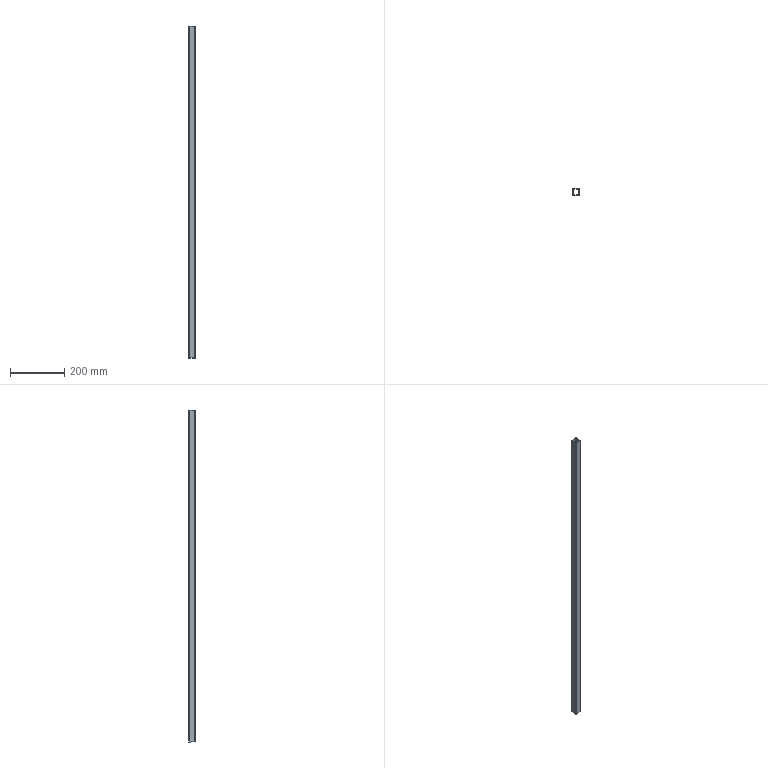Part | SolidWorks | features Extrusion 1 | 1 solid | 18 faces | box 25 x 25 x 1224 mm | volume 212608 mm3 | plane 10 | cylinder 8 | commonest cylinder face diameters 4 x4 8 x4
STEP:
#1=CARTESIAN_POINT('',(12.5,8.5,1224.));
#2=VERTEX_POINT('',#1);
#3=CARTESIAN_POINT('',(8.5,12.5,1224.));
#4=VERTEX_POINT('',#3);
#5=CARTESIAN_POINT('',(8.5,8.5,1224.));
#6=DIRECTION('',(0.,0.,1.));
#7=DIRECTION('',(1.,0.,0.));
#8=AXIS2_PLACEMENT_3D('',#5,#6,#7);
#9=CIRCLE('',#8,4.);
#10=EDGE_CURVE('',#2,#4,#9,.T.);
#11=ORIENTED_EDGE('',*,*,#10,.T.);
#12=CARTESIAN_POINT('',(-8.5,12.5,1224.));
#13=VERTEX_POINT('',#12);
#14=CARTESIAN_POINT('',(8.5,12.5,1224.));
#15=DIRECTION('',(-1.,0.,0.));
#16=VECTOR('',#15,1000.);
#17=LINE('',#14,#16);
#18=EDGE_CURVE('',#4,#13,#17,.T.);
#19=ORIENTED_EDGE('',*,*,#18,.T.);
#20=CARTESIAN_POINT('',(-12.5,8.5,1224.));
#21=VERTEX_POINT('',#20);
#22=CARTESIAN_POINT('',(-8.5,8.5,1224.));
#23=DIRECTION('',(0.,0.,1.));
#24=DIRECTION('',(1.,0.,0.));
#25=AXIS2_PLACEMENT_3D('',#22,#23,#24);
#26=CIRCLE('',#25,4.);
#27=EDGE_CURVE('',#13,#21,#26,.T.);
#28=ORIENTED_EDGE('',*,*,#27,.T.);
#29=CARTESIAN_POINT('',(-12.5,-8.5,1224.));
#30=VERTEX_POINT('',#29);
#31=CARTESIAN_POINT('',(-12.5,-8.5,1224.));
#32=DIRECTION('',(0.,-1.,0.));
#33=VECTOR('',#32,1000.);
#34=LINE('',#31,#33);
#35=EDGE_CURVE('',#21,#30,#34,.T.);
#36=ORIENTED_EDGE('',*,*,#35,.T.);
#37=CARTESIAN_POINT('',(-8.5,-12.5,1224.));
#38=VERTEX_POINT('',#37);
#39=CARTESIAN_POINT('',(-8.5,-8.5,1224.));
#40=DIRECTION('',(0.,0.,1.));
#41=DIRECTION('',(1.,0.,0.));
#42=AXIS2_PLACEMENT_3D('',#39,#40,#41);
#43=CIRCLE('',#42,4.);
#44=EDGE_CURVE('',#30,#38,#43,.T.);
#45=ORIENTED_EDGE('',*,*,#44,.T.);
#46=CARTESIAN_POINT('',(8.5,-12.5,1224.));
#47=VERTEX_POINT('',#46);
#48=CARTESIAN_POINT('',(-8.5,-12.5,1224.));
#49=DIRECTION('',(1.,0.,0.));
#50=VECTOR('',#49,1000.);
#51=LINE('',#48,#50);
#52=EDGE_CURVE('',#38,#47,#51,.T.);
#53=ORIENTED_EDGE('',*,*,#52,.T.);
#54=CARTESIAN_POINT('',(12.5,-8.5,1224.));
#55=VERTEX_POINT('',#54);
#56=CARTESIAN_POINT('',(8.5,-8.5,1224.));
#57=DIRECTION('',(0.,0.,1.));
#58=DIRECTION('',(1.,0.,0.));
#59=AXIS2_PLACEMENT_3D('',#56,#57,#58);
#60=CIRCLE('',#59,4.);
#61=EDGE_CURVE('',#47,#55,#60,.T.);
#62=ORIENTED_EDGE('',*,*,#61,.T.);
#63=CARTESIAN_POINT('',(12.5,8.5,1224.));
#64=DIRECTION('',(0.,1.,0.));
#65=VECTOR('',#64,1000.);
#66=LINE('',#63,#65);
#67=EDGE_CURVE('',#55,#2,#66,.T.);
#68=ORIENTED_EDGE('',*,*,#67,.T.);
#69=EDGE_LOOP('',(#11,#19,#28,#36,#45,#53,#62,#68));
#70=FACE_OUTER_BOUND('',#69,.T.);
#71=CARTESIAN_POINT('',(-10.5,8.5,1224.));
#72=VERTEX_POINT('',#71);
#73=CARTESIAN_POINT('',(-10.5,-8.5,1224.));
#74=VERTEX_POINT('',#73);
#75=CARTESIAN_POINT('',(-10.5,-8.5,1224.));
#76=DIRECTION('',(0.,-1.,0.));
#77=VECTOR('',#76,1000.);
#78=LINE('',#75,#77);
#79=EDGE_CURVE('',#72,#74,#78,.T.);
#80=ORIENTED_EDGE('',*,*,#79,.F.);
#81=CARTESIAN_POINT('',(-8.5,10.5,1224.));
#82=VERTEX_POINT('',#81);
#83=CARTESIAN_POINT('',(-8.5,8.5,1224.));
#84=DIRECTION('',(0.,0.,1.));
#85=DIRECTION('',(1.,0.,0.));
#86=AXIS2_PLACEMENT_3D('',#83,#84,#85);
#87=CIRCLE('',#86,2.);
#88=EDGE_CURVE('',#82,#72,#87,.T.);
#89=ORIENTED_EDGE('',*,*,#88,.F.);
#90=CARTESIAN_POINT('',(8.5,10.5,1224.));
#91=VERTEX_POINT('',#90);
#92=CARTESIAN_POINT('',(8.5,10.5,1224.));
#93=DIRECTION('',(-1.,0.,0.));
#94=VECTOR('',#93,1000.);
#95=LINE('',#92,#94);
#96=EDGE_CURVE('',#91,#82,#95,.T.);
#97=ORIENTED_EDGE('',*,*,#96,.F.);
#98=CARTESIAN_POINT('',(10.5,8.5,1224.));
#99=VERTEX_POINT('',#98);
#100=CARTESIAN_POINT('',(8.5,8.5,1224.));
#101=DIRECTION('',(0.,0.,1.));
#102=DIRECTION('',(1.,0.,0.));
#103=AXIS2_PLACEMENT_3D('',#100,#101,#102);
#104=CIRCLE('',#103,2.);
#105=EDGE_CURVE('',#99,#91,#104,.T.);
#106=ORIENTED_EDGE('',*,*,#105,.F.);
#107=CARTESIAN_POINT('',(10.5,-8.5,1224.));
#108=VERTEX_POINT('',#107);
#109=CARTESIAN_POINT('',(10.5,8.5,1224.));
#110=DIRECTION('',(0.,1.,0.));
#111=VECTOR('',#110,1000.);
#112=LINE('',#109,#111);
#113=EDGE_CURVE('',#108,#99,#112,.T.);
#114=ORIENTED_EDGE('',*,*,#113,.F.);
#115=CARTESIAN_POINT('',(8.5,-10.5,1224.));
#116=VERTEX_POINT('',#115);
#117=CARTESIAN_POINT('',(8.5,-8.5,1224.));
#118=DIRECTION('',(0.,0.,1.));
#119=DIRECTION('',(1.,0.,0.));
#120=AXIS2_PLACEMENT_3D('',#117,#118,#119);
#121=CIRCLE('',#120,2.);
#122=EDGE_CURVE('',#116,#108,#121,.T.);
#123=ORIENTED_EDGE('',*,*,#122,.F.);
#124=CARTESIAN_POINT('',(-8.5,-10.5,1224.));
#125=VERTEX_POINT('',#124);
#126=CARTESIAN_POINT('',(-8.5,-10.5,1224.));
#127=DIRECTION('',(1.,0.,0.));
#128=VECTOR('',#127,1000.);
#129=LINE('',#126,#128);
#130=EDGE_CURVE('',#125,#116,#129,.T.);
#131=ORIENTED_EDGE('',*,*,#130,.F.);
#132=CARTESIAN_POINT('',(-8.5,-8.5,1224.));
#133=DIRECTION('',(0.,0.,1.));
#134=DIRECTION('',(1.,0.,0.));
#135=AXIS2_PLACEMENT_3D('',#132,#133,#134);
#136=CIRCLE('',#135,2.);
#137=EDGE_CURVE('',#74,#125,#136,.T.);
#138=ORIENTED_EDGE('',*,*,#137,.F.);
#139=EDGE_LOOP('',(#80,#89,#97,#106,#114,#123,#131,#138));
#140=FACE_BOUND('',#139,.T.);
#141=CARTESIAN_POINT('',(8.5,8.5,1224.));
#142=DIRECTION('',(0.,0.,1.));
#143=DIRECTION('',(1.,0.,0.));
#144=AXIS2_PLACEMENT_3D('',#141,#142,#143);
#145=PLANE('',#144);
#146=ADVANCED_FACE('',(#70,#140),#145,.T.);
#147=CARTESIAN_POINT('',(12.5,8.5,0.));
#148=VERTEX_POINT('',#147);
#149=CARTESIAN_POINT('',(8.5,12.5,0.));
#150=VERTEX_POINT('',#149);
#151=CARTESIAN_POINT('',(8.5,8.5,0.));
#152=DIRECTION('',(0.,0.,1.));
#153=DIRECTION('',(1.,0.,0.));
#154=AXIS2_PLACEMENT_3D('',#151,#152,#153);
#155=CIRCLE('',#154,4.);
#156=EDGE_CURVE('',#148,#150,#155,.T.);
#157=ORIENTED_EDGE('',*,*,#156,.F.);
#158=CARTESIAN_POINT('',(12.5,-8.5,0.));
#159=VERTEX_POINT('',#158);
#160=CARTESIAN_POINT('',(12.5,8.5,0.));
#161=DIRECTION('',(0.,1.,0.));
#162=VECTOR('',#161,1000.);
#163=LINE('',#160,#162);
#164=EDGE_CURVE('',#159,#148,#163,.T.);
#165=ORIENTED_EDGE('',*,*,#164,.F.);
#166=CARTESIAN_POINT('',(8.5,-12.5,0.));
#167=VERTEX_POINT('',#166);
#168=CARTESIAN_POINT('',(8.5,-8.5,0.));
#169=DIRECTION('',(0.,0.,1.));
#170=DIRECTION('',(1.,0.,0.));
#171=AXIS2_PLACEMENT_3D('',#168,#169,#170);
#172=CIRCLE('',#171,4.);
#173=EDGE_CURVE('',#167,#159,#172,.T.);
#174=ORIENTED_EDGE('',*,*,#173,.F.);
#175=CARTESIAN_POINT('',(-8.5,-12.5,0.));
#176=VERTEX_POINT('',#175);
#177=CARTESIAN_POINT('',(-8.5,-12.5,0.));
#178=DIRECTION('',(1.,0.,0.));
#179=VECTOR('',#178,1000.);
#180=LINE('',#177,#179);
#181=EDGE_CURVE('',#176,#167,#180,.T.);
#182=ORIENTED_EDGE('',*,*,#181,.F.);
#183=CARTESIAN_POINT('',(-12.5,-8.5,0.));
#184=VERTEX_POINT('',#183);
#185=CARTESIAN_POINT('',(-8.5,-8.5,0.));
#186=DIRECTION('',(0.,0.,1.));
#187=DIRECTION('',(1.,0.,0.));
#188=AXIS2_PLACEMENT_3D('',#185,#186,#187);
#189=CIRCLE('',#188,4.);
#190=EDGE_CURVE('',#184,#176,#189,.T.);
#191=ORIENTED_EDGE('',*,*,#190,.F.);
#192=CARTESIAN_POINT('',(-12.5,8.5,0.));
#193=VERTEX_POINT('',#192);
#194=CARTESIAN_POINT('',(-12.5,-8.5,0.));
#195=DIRECTION('',(0.,-1.,0.));
#196=VECTOR('',#195,1000.);
#197=LINE('',#194,#196);
#198=EDGE_CURVE('',#193,#184,#197,.T.);
#199=ORIENTED_EDGE('',*,*,#198,.F.);
#200=CARTESIAN_POINT('',(-8.5,12.5,0.));
#201=VERTEX_POINT('',#200);
#202=CARTESIAN_POINT('',(-8.5,8.5,0.));
#203=DIRECTION('',(0.,0.,1.));
#204=DIRECTION('',(1.,0.,0.));
#205=AXIS2_PLACEMENT_3D('',#202,#203,#204);
#206=CIRCLE('',#205,4.);
#207=EDGE_CURVE('',#201,#193,#206,.T.);
#208=ORIENTED_EDGE('',*,*,#207,.F.);
#209=CARTESIAN_POINT('',(8.5,12.5,0.));
#210=DIRECTION('',(-1.,0.,0.));
#211=VECTOR('',#210,1000.);
#212=LINE('',#209,#211);
#213=EDGE_CURVE('',#150,#201,#212,.T.);
#214=ORIENTED_EDGE('',*,*,#213,.F.);
#215=EDGE_LOOP('',(#157,#165,#174,#182,#191,#199,#208,#214));
#216=FACE_OUTER_BOUND('',#215,.T.);
#217=CARTESIAN_POINT('',(-8.5,10.5,0.));
#218=VERTEX_POINT('',#217);
#219=CARTESIAN_POINT('',(-10.5,8.5,0.));
#220=VERTEX_POINT('',#219);
#221=CARTESIAN_POINT('',(-8.5,8.5,0.));
#222=DIRECTION('',(0.,0.,1.));
#223=DIRECTION('',(1.,0.,0.));
#224=AXIS2_PLACEMENT_3D('',#221,#222,#223);
#225=CIRCLE('',#224,2.);
#226=EDGE_CURVE('',#218,#220,#225,.T.);
#227=ORIENTED_EDGE('',*,*,#226,.T.);
#228=CARTESIAN_POINT('',(-10.5,-8.5,0.));
#229=VERTEX_POINT('',#228);
#230=CARTESIAN_POINT('',(-10.5,-8.5,0.));
#231=DIRECTION('',(0.,-1.,0.));
#232=VECTOR('',#231,1000.);
#233=LINE('',#230,#232);
#234=EDGE_CURVE('',#220,#229,#233,.T.);
#235=ORIENTED_EDGE('',*,*,#234,.T.);
#236=CARTESIAN_POINT('',(-8.5,-10.5,0.));
#237=VERTEX_POINT('',#236);
#238=CARTESIAN_POINT('',(-8.5,-8.5,0.));
#239=DIRECTION('',(0.,0.,1.));
#240=DIRECTION('',(1.,0.,0.));
#241=AXIS2_PLACEMENT_3D('',#238,#239,#240);
#242=CIRCLE('',#241,2.);
#243=EDGE_CURVE('',#229,#237,#242,.T.);
#244=ORIENTED_EDGE('',*,*,#243,.T.);
#245=CARTESIAN_POINT('',(8.5,-10.5,0.));
#246=VERTEX_POINT('',#245);
#247=CARTESIAN_POINT('',(-8.5,-10.5,0.));
#248=DIRECTION('',(1.,0.,0.));
#249=VECTOR('',#248,1000.);
#250=LINE('',#247,#249);
#251=EDGE_CURVE('',#237,#246,#250,.T.);
#252=ORIENTED_EDGE('',*,*,#251,.T.);
#253=CARTESIAN_POINT('',(10.5,-8.5,0.));
#254=VERTEX_POINT('',#253);
#255=CARTESIAN_POINT('',(8.5,-8.5,0.));
#256=DIRECTION('',(0.,0.,1.));
#257=DIRECTION('',(1.,0.,0.));
#258=AXIS2_PLACEMENT_3D('',#255,#256,#257);
#259=CIRCLE('',#258,2.);
#260=EDGE_CURVE('',#246,#254,#259,.T.);
#261=ORIENTED_EDGE('',*,*,#260,.T.);
#262=CARTESIAN_POINT('',(10.5,8.5,0.));
#263=VERTEX_POINT('',#262);
#264=CARTESIAN_POINT('',(10.5,8.5,0.));
#265=DIRECTION('',(0.,1.,0.));
#266=VECTOR('',#265,1000.);
#267=LINE('',#264,#266);
#268=EDGE_CURVE('',#254,#263,#267,.T.);
#269=ORIENTED_EDGE('',*,*,#268,.T.);
#270=CARTESIAN_POINT('',(8.5,10.5,0.));
#271=VERTEX_POINT('',#270);
#272=CARTESIAN_POINT('',(8.5,8.5,0.));
#273=DIRECTION('',(0.,0.,1.));
#274=DIRECTION('',(1.,0.,0.));
#275=AXIS2_PLACEMENT_3D('',#272,#273,#274);
#276=CIRCLE('',#275,2.);
#277=EDGE_CURVE('',#263,#271,#276,.T.);
#278=ORIENTED_EDGE('',*,*,#277,.T.);
#279=CARTESIAN_POINT('',(8.5,10.5,0.));
#280=DIRECTION('',(-1.,0.,0.));
#281=VECTOR('',#280,1000.);
#282=LINE('',#279,#281);
#283=EDGE_CURVE('',#271,#218,#282,.T.);
#284=ORIENTED_EDGE('',*,*,#283,.T.);
#285=EDGE_LOOP('',(#227,#235,#244,#252,#261,#269,#278,#284));
#286=FACE_BOUND('',#285,.T.);
#287=CARTESIAN_POINT('',(8.5,8.5,0.));
#288=DIRECTION('',(0.,0.,1.));
#289=DIRECTION('',(1.,0.,0.));
#290=AXIS2_PLACEMENT_3D('',#287,#288,#289);
#291=PLANE('',#290);
#292=ADVANCED_FACE('',(#216,#286),#291,.F.);
#293=ORIENTED_EDGE('',*,*,#156,.T.);
#294=CARTESIAN_POINT('',(8.5,12.5,1224.));
#295=DIRECTION('',(0.,0.,-1.));
#296=VECTOR('',#295,1000.);
#297=LINE('',#294,#296);
#298=EDGE_CURVE('',#4,#150,#297,.T.);
#299=ORIENTED_EDGE('',*,*,#298,.F.);
#300=ORIENTED_EDGE('',*,*,#10,.F.);
#301=CARTESIAN_POINT('',(12.5,8.5,1224.));
#302=DIRECTION('',(0.,0.,-1.));
#303=VECTOR('',#302,1000.);
#304=LINE('',#301,#303);
#305=EDGE_CURVE('',#2,#148,#304,.T.);
#306=ORIENTED_EDGE('',*,*,#305,.T.);
#307=EDGE_LOOP('',(#293,#299,#300,#306));
#308=FACE_OUTER_BOUND('',#307,.T.);
#309=CARTESIAN_POINT('',(8.5,8.5,1224.));
#310=DIRECTION('',(0.,0.,-1.));
#311=DIRECTION('',(-1.,0.,0.));
#312=AXIS2_PLACEMENT_3D('',#309,#310,#311);
#313=CYLINDRICAL_SURFACE('',#312,4.);
#314=ADVANCED_FACE('',(#308),#313,.T.);
#315=ORIENTED_EDGE('',*,*,#213,.T.);
#316=CARTESIAN_POINT('',(-8.5,12.5,1224.));
#317=DIRECTION('',(0.,0.,-1.));
#318=VECTOR('',#317,1000.);
#319=LINE('',#316,#318);
#320=EDGE_CURVE('',#13,#201,#319,.T.);
#321=ORIENTED_EDGE('',*,*,#320,.F.);
#322=ORIENTED_EDGE('',*,*,#18,.F.);
#323=ORIENTED_EDGE('',*,*,#298,.T.);
#324=EDGE_LOOP('',(#315,#321,#322,#323));
#325=FACE_OUTER_BOUND('',#324,.T.);
#326=CARTESIAN_POINT('',(8.5,12.5,1224.));
#327=DIRECTION('',(0.,-1.,0.));
#328=DIRECTION('',(0.,0.,-1.));
#329=AXIS2_PLACEMENT_3D('',#326,#327,#328);
#330=PLANE('',#329);
#331=ADVANCED_FACE('',(#325),#330,.F.);
#332=ORIENTED_EDGE('',*,*,#207,.T.);
#333=CARTESIAN_POINT('',(-12.5,8.5,1224.));
#334=DIRECTION('',(0.,0.,-1.));
#335=VECTOR('',#334,1000.);
#336=LINE('',#333,#335);
#337=EDGE_CURVE('',#21,#193,#336,.T.);
#338=ORIENTED_EDGE('',*,*,#337,.F.);
#339=ORIENTED_EDGE('',*,*,#27,.F.);
#340=ORIENTED_EDGE('',*,*,#320,.T.);
#341=EDGE_LOOP('',(#332,#338,#339,#340));
#342=FACE_OUTER_BOUND('',#341,.T.);
#343=CARTESIAN_POINT('',(-8.5,8.5,1224.));
#344=DIRECTION('',(0.,0.,-1.));
#345=DIRECTION('',(-1.,0.,0.));
#346=AXIS2_PLACEMENT_3D('',#343,#344,#345);
#347=CYLINDRICAL_SURFACE('',#346,4.);
#348=ADVANCED_FACE('',(#342),#347,.T.);
#349=ORIENTED_EDGE('',*,*,#198,.T.);
#350=CARTESIAN_POINT('',(-12.5,-8.5,1224.));
#351=DIRECTION('',(0.,0.,-1.));
#352=VECTOR('',#351,1000.);
#353=LINE('',#350,#352);
#354=EDGE_CURVE('',#30,#184,#353,.T.);
#355=ORIENTED_EDGE('',*,*,#354,.F.);
#356=ORIENTED_EDGE('',*,*,#35,.F.);
#357=ORIENTED_EDGE('',*,*,#337,.T.);
#358=EDGE_LOOP('',(#349,#355,#356,#357));
#359=FACE_OUTER_BOUND('',#358,.T.);
#360=CARTESIAN_POINT('',(-12.5,-8.5,1224.));
#361=DIRECTION('',(1.,0.,0.));
#362=DIRECTION('',(0.,0.,-1.));
#363=AXIS2_PLACEMENT_3D('',#360,#361,#362);
#364=PLANE('',#363);
#365=ADVANCED_FACE('',(#359),#364,.F.);
#366=ORIENTED_EDGE('',*,*,#190,.T.);
#367=CARTESIAN_POINT('',(-8.5,-12.5,1224.));
#368=DIRECTION('',(0.,0.,-1.));
#369=VECTOR('',#368,1000.);
#370=LINE('',#367,#369);
#371=EDGE_CURVE('',#38,#176,#370,.T.);
#372=ORIENTED_EDGE('',*,*,#371,.F.);
#373=ORIENTED_EDGE('',*,*,#44,.F.);
#374=ORIENTED_EDGE('',*,*,#354,.T.);
#375=EDGE_LOOP('',(#366,#372,#373,#374));
#376=FACE_OUTER_BOUND('',#375,.T.);
#377=CARTESIAN_POINT('',(-8.5,-8.5,1224.));
#378=DIRECTION('',(0.,0.,-1.));
#379=DIRECTION('',(-1.,0.,0.));
#380=AXIS2_PLACEMENT_3D('',#377,#378,#379);
#381=CYLINDRICAL_SURFACE('',#380,4.);
#382=ADVANCED_FACE('',(#376),#381,.T.);
#383=ORIENTED_EDGE('',*,*,#181,.T.);
#384=CARTESIAN_POINT('',(8.5,-12.5,1224.));
#385=DIRECTION('',(0.,0.,-1.));
#386=VECTOR('',#385,1000.);
#387=LINE('',#384,#386);
#388=EDGE_CURVE('',#47,#167,#387,.T.);
#389=ORIENTED_EDGE('',*,*,#388,.F.);
#390=ORIENTED_EDGE('',*,*,#52,.F.);
#391=ORIENTED_EDGE('',*,*,#371,.T.);
#392=EDGE_LOOP('',(#383,#389,#390,#391));
#393=FACE_OUTER_BOUND('',#392,.T.);
#394=CARTESIAN_POINT('',(-8.5,-12.5,1224.));
#395=DIRECTION('',(0.,1.,0.));
#396=DIRECTION('',(0.,0.,1.));
#397=AXIS2_PLACEMENT_3D('',#394,#395,#396);
#398=PLANE('',#397);
#399=ADVANCED_FACE('',(#393),#398,.F.);
#400=ORIENTED_EDGE('',*,*,#173,.T.);
#401=CARTESIAN_POINT('',(12.5,-8.5,1224.));
#402=DIRECTION('',(0.,0.,-1.));
#403=VECTOR('',#402,1000.);
#404=LINE('',#401,#403);
#405=EDGE_CURVE('',#55,#159,#404,.T.);
#406=ORIENTED_EDGE('',*,*,#405,.F.);
#407=ORIENTED_EDGE('',*,*,#61,.F.);
#408=ORIENTED_EDGE('',*,*,#388,.T.);
#409=EDGE_LOOP('',(#400,#406,#407,#408));
#410=FACE_OUTER_BOUND('',#409,.T.);
#411=CARTESIAN_POINT('',(8.5,-8.5,1224.));
#412=DIRECTION('',(0.,0.,-1.));
#413=DIRECTION('',(-1.,0.,0.));
#414=AXIS2_PLACEMENT_3D('',#411,#412,#413);
#415=CYLINDRICAL_SURFACE('',#414,4.);
#416=ADVANCED_FACE('',(#410),#415,.T.);
#417=ORIENTED_EDGE('',*,*,#164,.T.);
#418=ORIENTED_EDGE('',*,*,#305,.F.);
#419=ORIENTED_EDGE('',*,*,#67,.F.);
#420=ORIENTED_EDGE('',*,*,#405,.T.);
#421=EDGE_LOOP('',(#417,#418,#419,#420));
#422=FACE_OUTER_BOUND('',#421,.T.);
#423=CARTESIAN_POINT('',(12.5,8.5,1224.));
#424=DIRECTION('',(-1.,0.,0.));
#425=DIRECTION('',(0.,0.,1.));
#426=AXIS2_PLACEMENT_3D('',#423,#424,#425);
#427=PLANE('',#426);
#428=ADVANCED_FACE('',(#422),#427,.F.);
#429=ORIENTED_EDGE('',*,*,#226,.F.);
#430=CARTESIAN_POINT('',(-8.5,10.5,1224.));
#431=DIRECTION('',(0.,0.,-1.));
#432=VECTOR('',#431,1000.);
#433=LINE('',#430,#432);
#434=EDGE_CURVE('',#82,#218,#433,.T.);
#435=ORIENTED_EDGE('',*,*,#434,.F.);
#436=ORIENTED_EDGE('',*,*,#88,.T.);
#437=CARTESIAN_POINT('',(-10.5,8.5,1224.));
#438=DIRECTION('',(0.,0.,-1.));
#439=VECTOR('',#438,1000.);
#440=LINE('',#437,#439);
#441=EDGE_CURVE('',#72,#220,#440,.T.);
#442=ORIENTED_EDGE('',*,*,#441,.T.);
#443=EDGE_LOOP('',(#429,#435,#436,#442));
#444=FACE_OUTER_BOUND('',#443,.T.);
#445=CARTESIAN_POINT('',(-8.5,8.5,1224.));
#446=DIRECTION('',(0.,0.,-1.));
#447=DIRECTION('',(-1.,0.,0.));
#448=AXIS2_PLACEMENT_3D('',#445,#446,#447);
#449=CYLINDRICAL_SURFACE('',#448,2.);
#450=ADVANCED_FACE('',(#444),#449,.F.);
#451=ORIENTED_EDGE('',*,*,#234,.F.);
#452=ORIENTED_EDGE('',*,*,#441,.F.);
#453=ORIENTED_EDGE('',*,*,#79,.T.);
#454=CARTESIAN_POINT('',(-10.5,-8.5,1224.));
#455=DIRECTION('',(0.,0.,-1.));
#456=VECTOR('',#455,1000.);
#457=LINE('',#454,#456);
#458=EDGE_CURVE('',#74,#229,#457,.T.);
#459=ORIENTED_EDGE('',*,*,#458,.T.);
#460=EDGE_LOOP('',(#451,#452,#453,#459));
#461=FACE_OUTER_BOUND('',#460,.T.);
#462=CARTESIAN_POINT('',(-10.5,-8.5,1224.));
#463=DIRECTION('',(1.,0.,0.));
#464=DIRECTION('',(0.,0.,-1.));
#465=AXIS2_PLACEMENT_3D('',#462,#463,#464);
#466=PLANE('',#465);
#467=ADVANCED_FACE('',(#461),#466,.T.);
#468=ORIENTED_EDGE('',*,*,#243,.F.);
#469=ORIENTED_EDGE('',*,*,#458,.F.);
#470=ORIENTED_EDGE('',*,*,#137,.T.);
#471=CARTESIAN_POINT('',(-8.5,-10.5,1224.));
#472=DIRECTION('',(0.,0.,-1.));
#473=VECTOR('',#472,1000.);
#474=LINE('',#471,#473);
#475=EDGE_CURVE('',#125,#237,#474,.T.);
#476=ORIENTED_EDGE('',*,*,#475,.T.);
#477=EDGE_LOOP('',(#468,#469,#470,#476));
#478=FACE_OUTER_BOUND('',#477,.T.);
#479=CARTESIAN_POINT('',(-8.5,-8.5,1224.));
#480=DIRECTION('',(0.,0.,-1.));
#481=DIRECTION('',(-1.,0.,0.));
#482=AXIS2_PLACEMENT_3D('',#479,#480,#481);
#483=CYLINDRICAL_SURFACE('',#482,2.);
#484=ADVANCED_FACE('',(#478),#483,.F.);
#485=ORIENTED_EDGE('',*,*,#251,.F.);
#486=ORIENTED_EDGE('',*,*,#475,.F.);
#487=ORIENTED_EDGE('',*,*,#130,.T.);
#488=CARTESIAN_POINT('',(8.5,-10.5,1224.));
#489=DIRECTION('',(0.,0.,-1.));
#490=VECTOR('',#489,1000.);
#491=LINE('',#488,#490);
#492=EDGE_CURVE('',#116,#246,#491,.T.);
#493=ORIENTED_EDGE('',*,*,#492,.T.);
#494=EDGE_LOOP('',(#485,#486,#487,#493));
#495=FACE_OUTER_BOUND('',#494,.T.);
#496=CARTESIAN_POINT('',(-8.5,-10.5,1224.));
#497=DIRECTION('',(0.,1.,0.));
#498=DIRECTION('',(0.,0.,1.));
#499=AXIS2_PLACEMENT_3D('',#496,#497,#498);
#500=PLANE('',#499);
#501=ADVANCED_FACE('',(#495),#500,.T.);
#502=ORIENTED_EDGE('',*,*,#260,.F.);
#503=ORIENTED_EDGE('',*,*,#492,.F.);
#504=ORIENTED_EDGE('',*,*,#122,.T.);
#505=CARTESIAN_POINT('',(10.5,-8.5,1224.));
#506=DIRECTION('',(0.,0.,-1.));
#507=VECTOR('',#506,1000.);
#508=LINE('',#505,#507);
#509=EDGE_CURVE('',#108,#254,#508,.T.);
#510=ORIENTED_EDGE('',*,*,#509,.T.);
#511=EDGE_LOOP('',(#502,#503,#504,#510));
#512=FACE_OUTER_BOUND('',#511,.T.);
#513=CARTESIAN_POINT('',(8.5,-8.5,1224.));
#514=DIRECTION('',(0.,0.,-1.));
#515=DIRECTION('',(-1.,0.,0.));
#516=AXIS2_PLACEMENT_3D('',#513,#514,#515);
#517=CYLINDRICAL_SURFACE('',#516,2.);
#518=ADVANCED_FACE('',(#512),#517,.F.);
#519=ORIENTED_EDGE('',*,*,#268,.F.);
#520=ORIENTED_EDGE('',*,*,#509,.F.);
#521=ORIENTED_EDGE('',*,*,#113,.T.);
#522=CARTESIAN_POINT('',(10.5,8.5,1224.));
#523=DIRECTION('',(0.,0.,-1.));
#524=VECTOR('',#523,1000.);
#525=LINE('',#522,#524);
#526=EDGE_CURVE('',#99,#263,#525,.T.);
#527=ORIENTED_EDGE('',*,*,#526,.T.);
#528=EDGE_LOOP('',(#519,#520,#521,#527));
#529=FACE_OUTER_BOUND('',#528,.T.);
#530=CARTESIAN_POINT('',(10.5,8.5,1224.));
#531=DIRECTION('',(-1.,0.,0.));
#532=DIRECTION('',(0.,0.,1.));
#533=AXIS2_PLACEMENT_3D('',#530,#531,#532);
#534=PLANE('',#533);
#535=ADVANCED_FACE('',(#529),#534,.T.);
#536=ORIENTED_EDGE('',*,*,#277,.F.);
#537=ORIENTED_EDGE('',*,*,#526,.F.);
#538=ORIENTED_EDGE('',*,*,#105,.T.);
#539=CARTESIAN_POINT('',(8.5,10.5,1224.));
#540=DIRECTION('',(0.,0.,-1.));
#541=VECTOR('',#540,1000.);
#542=LINE('',#539,#541);
#543=EDGE_CURVE('',#91,#271,#542,.T.);
#544=ORIENTED_EDGE('',*,*,#543,.T.);
#545=EDGE_LOOP('',(#536,#537,#538,#544));
#546=FACE_OUTER_BOUND('',#545,.T.);
#547=CARTESIAN_POINT('',(8.5,8.5,1224.));
#548=DIRECTION('',(0.,0.,-1.));
#549=DIRECTION('',(-1.,0.,0.));
#550=AXIS2_PLACEMENT_3D('',#547,#548,#549);
#551=CYLINDRICAL_SURFACE('',#550,2.);
#552=ADVANCED_FACE('',(#546),#551,.F.);
#553=ORIENTED_EDGE('',*,*,#283,.F.);
#554=ORIENTED_EDGE('',*,*,#543,.F.);
#555=ORIENTED_EDGE('',*,*,#96,.T.);
#556=ORIENTED_EDGE('',*,*,#434,.T.);
#557=EDGE_LOOP('',(#553,#554,#555,#556));
#558=FACE_OUTER_BOUND('',#557,.T.);
#559=CARTESIAN_POINT('',(8.5,10.5,1224.));
#560=DIRECTION('',(0.,-1.,0.));
#561=DIRECTION('',(0.,0.,-1.));
#562=AXIS2_PLACEMENT_3D('',#559,#560,#561);
#563=PLANE('',#562);
#564=ADVANCED_FACE('',(#558),#563,.T.);
#565=CLOSED_SHELL('',(#146,#292,#314,#331,#348,#365,#382,#399,#416,#428,#450,#467,#484,#501,#518,#535,#552,#564));
#566=MANIFOLD_SOLID_BREP('',#565);
#567=CARTESIAN_POINT('',(0.,0.,0.));
#568=DIRECTION('',(0.,0.,1.));
#569=DIRECTION('',(1.,0.,0.));
#570=AXIS2_PLACEMENT_3D('',#567,#568,#569);
#571=(LENGTH_UNIT()NAMED_UNIT(*)SI_UNIT(.MILLI.,.METRE.));
#572=UNCERTAINTY_MEASURE_WITH_UNIT(LENGTH_MEASURE(0.00001),#571,'','');
#573=(NAMED_UNIT(*)PLANE_ANGLE_UNIT()SI_UNIT($,.RADIAN.));
#574=(NAMED_UNIT(*)SI_UNIT($,.STERADIAN.)SOLID_ANGLE_UNIT());
#575=(GEOMETRIC_REPRESENTATION_CONTEXT(3)GLOBAL_UNCERTAINTY_ASSIGNED_CONTEXT((#572))GLOBAL_UNIT_ASSIGNED_CONTEXT((#571,#573,#574))REPRESENTATION_CONTEXT('',''));
#576=ADVANCED_BREP_SHAPE_REPRESENTATION('',(#566,#570),#575);